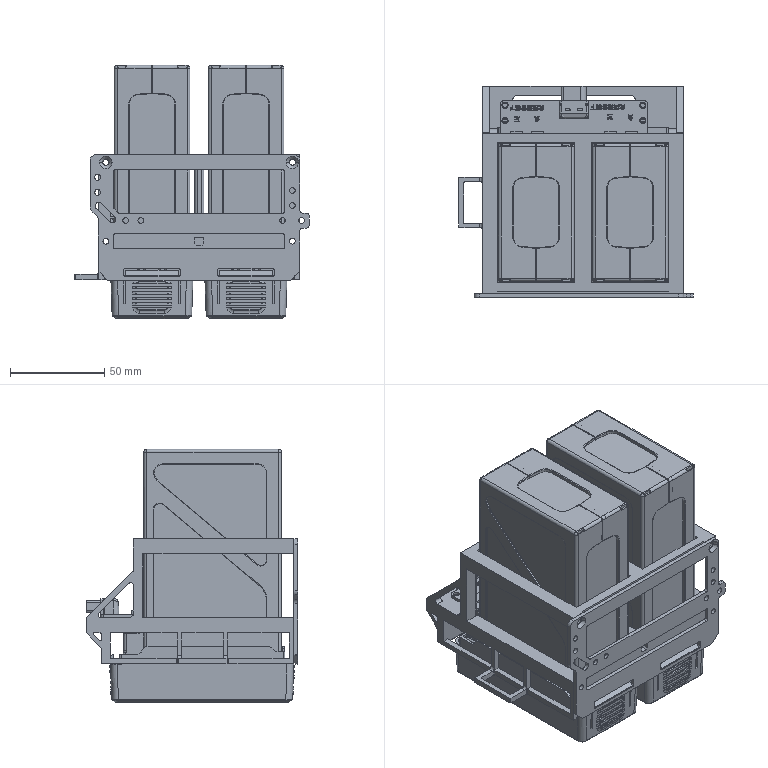Part | SolidWorks | features InContextFeatHolder 1 | 28 solids | 3913 faces | volume 914521 mm3 | plane 2520 | cylinder 986 | spline 207 | torus 118 | cone 58 | sphere 24 | commonest cylinder face diameters 1 x222 0.6 x136 2 x127 3 x74 4 x49 10 x44